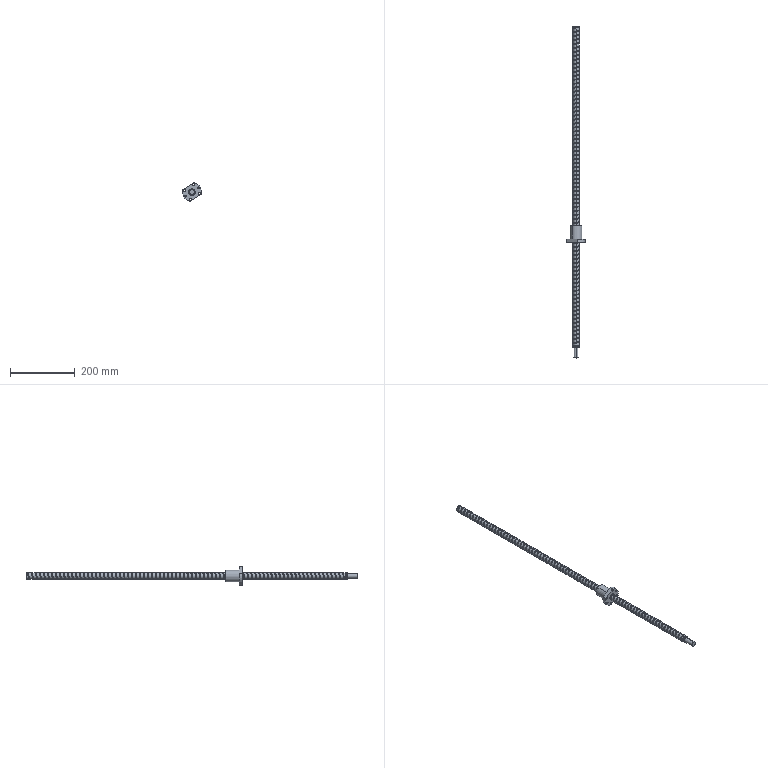Part | SolidWorks | features AEMSimFeature 1 | 2 solids | 231 faces | box 58 x 1028 x 57.544 mm | volume 346833 mm3 | cylinder 210 | plane 16 | spline 5 | commonest cylinder face diameters 20 x162 18 x21 5.5 x12 15 x8 19 x3 36 x2